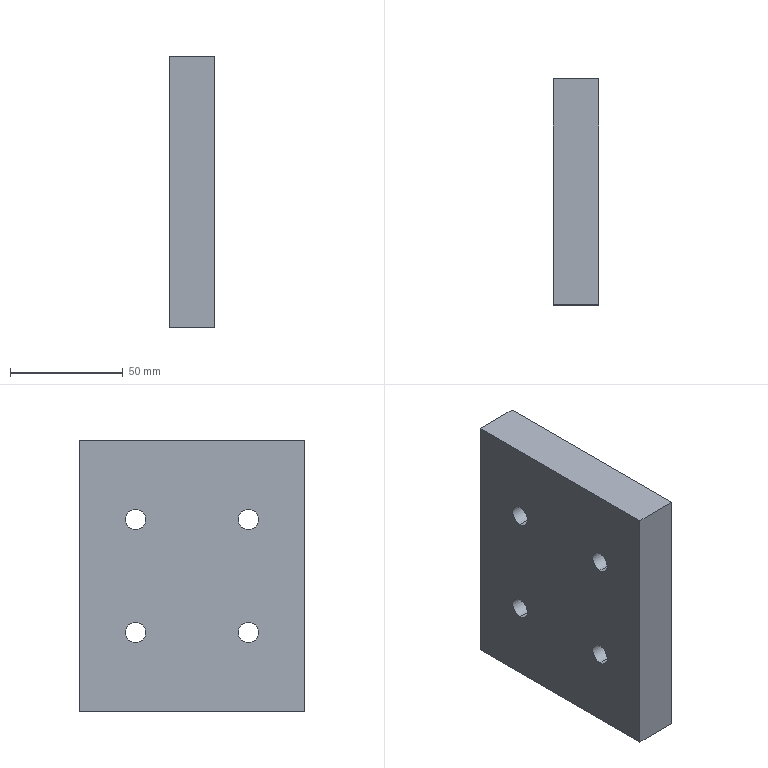Part | SolidWorks | features Extrusion 1, HoleWzd 1 | 1 solid | 14 faces | box 20 x 100 x 120 mm | volume 234911 mm3 | cylinder 8 | plane 6 | commonest cylinder face diameters 9 x8
STEP:
#1=CARTESIAN_POINT('',(0.,25.,29.5));
#2=VERTEX_POINT('',#1);
#3=CARTESIAN_POINT('',(0.,25.,20.5));
#4=VERTEX_POINT('',#3);
#5=CARTESIAN_POINT('',(0.,25.,25.));
#6=DIRECTION('',(1.,0.,0.));
#7=DIRECTION('',(0.,0.,-1.));
#8=AXIS2_PLACEMENT_3D('',#5,#6,#7);
#9=CIRCLE('',#8,4.5);
#10=EDGE_CURVE('',#2,#4,#9,.T.);
#11=ORIENTED_EDGE('',*,*,#10,.F.);
#12=CARTESIAN_POINT('',(20.,25.,29.5));
#13=VERTEX_POINT('',#12);
#14=CARTESIAN_POINT('',(20.,25.,29.5));
#15=DIRECTION('',(1.,0.,0.));
#16=VECTOR('',#15,1000.);
#17=LINE('',#14,#16);
#18=EDGE_CURVE('',#2,#13,#17,.T.);
#19=ORIENTED_EDGE('',*,*,#18,.T.);
#20=CARTESIAN_POINT('',(20.,25.,20.5));
#21=VERTEX_POINT('',#20);
#22=CARTESIAN_POINT('',(20.,25.,25.));
#23=DIRECTION('',(1.,0.,0.));
#24=DIRECTION('',(0.,0.,-1.));
#25=AXIS2_PLACEMENT_3D('',#22,#23,#24);
#26=CIRCLE('',#25,4.5);
#27=EDGE_CURVE('',#13,#21,#26,.T.);
#28=ORIENTED_EDGE('',*,*,#27,.T.);
#29=CARTESIAN_POINT('',(20.,25.,20.5));
#30=DIRECTION('',(1.,0.,0.));
#31=VECTOR('',#30,1000.);
#32=LINE('',#29,#31);
#33=EDGE_CURVE('',#4,#21,#32,.T.);
#34=ORIENTED_EDGE('',*,*,#33,.F.);
#35=EDGE_LOOP('',(#11,#19,#28,#34));
#36=FACE_OUTER_BOUND('',#35,.T.);
#37=CARTESIAN_POINT('',(20.,25.,25.));
#38=DIRECTION('',(1.,0.,0.));
#39=DIRECTION('',(0.,0.,-1.));
#40=AXIS2_PLACEMENT_3D('',#37,#38,#39);
#41=CYLINDRICAL_SURFACE('',#40,4.5);
#42=ADVANCED_FACE('',(#36),#41,.F.);
#43=CARTESIAN_POINT('',(0.,25.,-20.5));
#44=VERTEX_POINT('',#43);
#45=CARTESIAN_POINT('',(0.,25.,-29.5));
#46=VERTEX_POINT('',#45);
#47=CARTESIAN_POINT('',(0.,25.,-25.));
#48=DIRECTION('',(1.,0.,0.));
#49=DIRECTION('',(0.,0.,-1.));
#50=AXIS2_PLACEMENT_3D('',#47,#48,#49);
#51=CIRCLE('',#50,4.5);
#52=EDGE_CURVE('',#44,#46,#51,.T.);
#53=ORIENTED_EDGE('',*,*,#52,.F.);
#54=CARTESIAN_POINT('',(20.,25.,-20.5));
#55=VERTEX_POINT('',#54);
#56=CARTESIAN_POINT('',(20.,25.,-20.5));
#57=DIRECTION('',(1.,0.,0.));
#58=VECTOR('',#57,1000.);
#59=LINE('',#56,#58);
#60=EDGE_CURVE('',#44,#55,#59,.T.);
#61=ORIENTED_EDGE('',*,*,#60,.T.);
#62=CARTESIAN_POINT('',(20.,25.,-29.5));
#63=VERTEX_POINT('',#62);
#64=CARTESIAN_POINT('',(20.,25.,-25.));
#65=DIRECTION('',(1.,0.,0.));
#66=DIRECTION('',(0.,0.,-1.));
#67=AXIS2_PLACEMENT_3D('',#64,#65,#66);
#68=CIRCLE('',#67,4.5);
#69=EDGE_CURVE('',#55,#63,#68,.T.);
#70=ORIENTED_EDGE('',*,*,#69,.T.);
#71=CARTESIAN_POINT('',(20.,25.,-29.5));
#72=DIRECTION('',(1.,0.,0.));
#73=VECTOR('',#72,1000.);
#74=LINE('',#71,#73);
#75=EDGE_CURVE('',#46,#63,#74,.T.);
#76=ORIENTED_EDGE('',*,*,#75,.F.);
#77=EDGE_LOOP('',(#53,#61,#70,#76));
#78=FACE_OUTER_BOUND('',#77,.T.);
#79=CARTESIAN_POINT('',(20.,25.,-25.));
#80=DIRECTION('',(1.,0.,0.));
#81=DIRECTION('',(0.,0.,-1.));
#82=AXIS2_PLACEMENT_3D('',#79,#80,#81);
#83=CYLINDRICAL_SURFACE('',#82,4.5);
#84=ADVANCED_FACE('',(#78),#83,.F.);
#85=CARTESIAN_POINT('',(0.,-25.,29.5));
#86=VERTEX_POINT('',#85);
#87=CARTESIAN_POINT('',(0.,-25.,20.5));
#88=VERTEX_POINT('',#87);
#89=CARTESIAN_POINT('',(0.,-25.,25.));
#90=DIRECTION('',(1.,0.,0.));
#91=DIRECTION('',(0.,0.,-1.));
#92=AXIS2_PLACEMENT_3D('',#89,#90,#91);
#93=CIRCLE('',#92,4.5);
#94=EDGE_CURVE('',#86,#88,#93,.T.);
#95=ORIENTED_EDGE('',*,*,#94,.F.);
#96=CARTESIAN_POINT('',(20.,-25.,29.5));
#97=VERTEX_POINT('',#96);
#98=CARTESIAN_POINT('',(20.,-25.,29.5));
#99=DIRECTION('',(1.,0.,0.));
#100=VECTOR('',#99,1000.);
#101=LINE('',#98,#100);
#102=EDGE_CURVE('',#86,#97,#101,.T.);
#103=ORIENTED_EDGE('',*,*,#102,.T.);
#104=CARTESIAN_POINT('',(20.,-25.,20.5));
#105=VERTEX_POINT('',#104);
#106=CARTESIAN_POINT('',(20.,-25.,25.));
#107=DIRECTION('',(1.,0.,0.));
#108=DIRECTION('',(0.,0.,-1.));
#109=AXIS2_PLACEMENT_3D('',#106,#107,#108);
#110=CIRCLE('',#109,4.5);
#111=EDGE_CURVE('',#97,#105,#110,.T.);
#112=ORIENTED_EDGE('',*,*,#111,.T.);
#113=CARTESIAN_POINT('',(20.,-25.,20.5));
#114=DIRECTION('',(1.,0.,0.));
#115=VECTOR('',#114,1000.);
#116=LINE('',#113,#115);
#117=EDGE_CURVE('',#88,#105,#116,.T.);
#118=ORIENTED_EDGE('',*,*,#117,.F.);
#119=EDGE_LOOP('',(#95,#103,#112,#118));
#120=FACE_OUTER_BOUND('',#119,.T.);
#121=CARTESIAN_POINT('',(20.,-25.,25.));
#122=DIRECTION('',(1.,0.,0.));
#123=DIRECTION('',(0.,0.,-1.));
#124=AXIS2_PLACEMENT_3D('',#121,#122,#123);
#125=CYLINDRICAL_SURFACE('',#124,4.5);
#126=ADVANCED_FACE('',(#120),#125,.F.);
#127=CARTESIAN_POINT('',(0.,-25.,-20.5));
#128=VERTEX_POINT('',#127);
#129=CARTESIAN_POINT('',(0.,-25.,-29.5));
#130=VERTEX_POINT('',#129);
#131=CARTESIAN_POINT('',(0.,-25.,-25.));
#132=DIRECTION('',(1.,0.,0.));
#133=DIRECTION('',(0.,0.,-1.));
#134=AXIS2_PLACEMENT_3D('',#131,#132,#133);
#135=CIRCLE('',#134,4.5);
#136=EDGE_CURVE('',#128,#130,#135,.T.);
#137=ORIENTED_EDGE('',*,*,#136,.F.);
#138=CARTESIAN_POINT('',(20.,-25.,-20.5));
#139=VERTEX_POINT('',#138);
#140=CARTESIAN_POINT('',(20.,-25.,-20.5));
#141=DIRECTION('',(1.,0.,0.));
#142=VECTOR('',#141,1000.);
#143=LINE('',#140,#142);
#144=EDGE_CURVE('',#128,#139,#143,.T.);
#145=ORIENTED_EDGE('',*,*,#144,.T.);
#146=CARTESIAN_POINT('',(20.,-25.,-29.5));
#147=VERTEX_POINT('',#146);
#148=CARTESIAN_POINT('',(20.,-25.,-25.));
#149=DIRECTION('',(1.,0.,0.));
#150=DIRECTION('',(0.,0.,-1.));
#151=AXIS2_PLACEMENT_3D('',#148,#149,#150);
#152=CIRCLE('',#151,4.5);
#153=EDGE_CURVE('',#139,#147,#152,.T.);
#154=ORIENTED_EDGE('',*,*,#153,.T.);
#155=CARTESIAN_POINT('',(20.,-25.,-29.5));
#156=DIRECTION('',(1.,0.,0.));
#157=VECTOR('',#156,1000.);
#158=LINE('',#155,#157);
#159=EDGE_CURVE('',#130,#147,#158,.T.);
#160=ORIENTED_EDGE('',*,*,#159,.F.);
#161=EDGE_LOOP('',(#137,#145,#154,#160));
#162=FACE_OUTER_BOUND('',#161,.T.);
#163=CARTESIAN_POINT('',(20.,-25.,-25.));
#164=DIRECTION('',(1.,0.,0.));
#165=DIRECTION('',(0.,0.,-1.));
#166=AXIS2_PLACEMENT_3D('',#163,#164,#165);
#167=CYLINDRICAL_SURFACE('',#166,4.5);
#168=ADVANCED_FACE('',(#162),#167,.F.);
#169=CARTESIAN_POINT('',(0.,-50.,-60.));
#170=VERTEX_POINT('',#169);
#171=CARTESIAN_POINT('',(0.,50.,-60.));
#172=VERTEX_POINT('',#171);
#173=CARTESIAN_POINT('',(0.,50.,-60.));
#174=DIRECTION('',(0.,1.,0.));
#175=VECTOR('',#174,1000.);
#176=LINE('',#173,#175);
#177=EDGE_CURVE('',#170,#172,#176,.T.);
#178=ORIENTED_EDGE('',*,*,#177,.T.);
#179=CARTESIAN_POINT('',(20.,50.,-60.));
#180=VERTEX_POINT('',#179);
#181=CARTESIAN_POINT('',(20.,50.,-60.));
#182=DIRECTION('',(-1.,0.,0.));
#183=VECTOR('',#182,1000.);
#184=LINE('',#181,#183);
#185=EDGE_CURVE('',#180,#172,#184,.T.);
#186=ORIENTED_EDGE('',*,*,#185,.F.);
#187=CARTESIAN_POINT('',(20.,-50.,-60.));
#188=VERTEX_POINT('',#187);
#189=CARTESIAN_POINT('',(20.,50.,-60.));
#190=DIRECTION('',(0.,1.,0.));
#191=VECTOR('',#190,1000.);
#192=LINE('',#189,#191);
#193=EDGE_CURVE('',#188,#180,#192,.T.);
#194=ORIENTED_EDGE('',*,*,#193,.F.);
#195=CARTESIAN_POINT('',(20.,-50.,-60.));
#196=DIRECTION('',(-1.,0.,0.));
#197=VECTOR('',#196,1000.);
#198=LINE('',#195,#197);
#199=EDGE_CURVE('',#188,#170,#198,.T.);
#200=ORIENTED_EDGE('',*,*,#199,.T.);
#201=EDGE_LOOP('',(#178,#186,#194,#200));
#202=FACE_OUTER_BOUND('',#201,.T.);
#203=CARTESIAN_POINT('',(20.,50.,-60.));
#204=DIRECTION('',(0.,0.,1.));
#205=DIRECTION('',(0.,-1.,0.));
#206=AXIS2_PLACEMENT_3D('',#203,#204,#205);
#207=PLANE('',#206);
#208=ADVANCED_FACE('',(#202),#207,.F.);
#209=CARTESIAN_POINT('',(0.,50.,60.));
#210=VERTEX_POINT('',#209);
#211=CARTESIAN_POINT('',(0.,50.,60.));
#212=DIRECTION('',(0.,0.,1.));
#213=VECTOR('',#212,1000.);
#214=LINE('',#211,#213);
#215=EDGE_CURVE('',#172,#210,#214,.T.);
#216=ORIENTED_EDGE('',*,*,#215,.T.);
#217=CARTESIAN_POINT('',(20.,50.,60.));
#218=VERTEX_POINT('',#217);
#219=CARTESIAN_POINT('',(20.,50.,60.));
#220=DIRECTION('',(-1.,0.,0.));
#221=VECTOR('',#220,1000.);
#222=LINE('',#219,#221);
#223=EDGE_CURVE('',#218,#210,#222,.T.);
#224=ORIENTED_EDGE('',*,*,#223,.F.);
#225=CARTESIAN_POINT('',(20.,50.,60.));
#226=DIRECTION('',(0.,0.,1.));
#227=VECTOR('',#226,1000.);
#228=LINE('',#225,#227);
#229=EDGE_CURVE('',#180,#218,#228,.T.);
#230=ORIENTED_EDGE('',*,*,#229,.F.);
#231=ORIENTED_EDGE('',*,*,#185,.T.);
#232=EDGE_LOOP('',(#216,#224,#230,#231));
#233=FACE_OUTER_BOUND('',#232,.T.);
#234=CARTESIAN_POINT('',(20.,50.,60.));
#235=DIRECTION('',(0.,-1.,0.));
#236=DIRECTION('',(0.,0.,-1.));
#237=AXIS2_PLACEMENT_3D('',#234,#235,#236);
#238=PLANE('',#237);
#239=ADVANCED_FACE('',(#233),#238,.F.);
#240=CARTESIAN_POINT('',(0.,-50.,60.));
#241=VERTEX_POINT('',#240);
#242=CARTESIAN_POINT('',(0.,50.,60.));
#243=DIRECTION('',(0.,-1.,0.));
#244=VECTOR('',#243,1000.);
#245=LINE('',#242,#244);
#246=EDGE_CURVE('',#210,#241,#245,.T.);
#247=ORIENTED_EDGE('',*,*,#246,.T.);
#248=CARTESIAN_POINT('',(20.,-50.,60.));
#249=VERTEX_POINT('',#248);
#250=CARTESIAN_POINT('',(20.,-50.,60.));
#251=DIRECTION('',(-1.,0.,0.));
#252=VECTOR('',#251,1000.);
#253=LINE('',#250,#252);
#254=EDGE_CURVE('',#249,#241,#253,.T.);
#255=ORIENTED_EDGE('',*,*,#254,.F.);
#256=CARTESIAN_POINT('',(20.,50.,60.));
#257=DIRECTION('',(0.,-1.,0.));
#258=VECTOR('',#257,1000.);
#259=LINE('',#256,#258);
#260=EDGE_CURVE('',#218,#249,#259,.T.);
#261=ORIENTED_EDGE('',*,*,#260,.F.);
#262=ORIENTED_EDGE('',*,*,#223,.T.);
#263=EDGE_LOOP('',(#247,#255,#261,#262));
#264=FACE_OUTER_BOUND('',#263,.T.);
#265=CARTESIAN_POINT('',(20.,50.,60.));
#266=DIRECTION('',(0.,0.,-1.));
#267=DIRECTION('',(0.,1.,0.));
#268=AXIS2_PLACEMENT_3D('',#265,#266,#267);
#269=PLANE('',#268);
#270=ADVANCED_FACE('',(#264),#269,.F.);
#271=CARTESIAN_POINT('',(0.,-50.,60.));
#272=DIRECTION('',(0.,0.,-1.));
#273=VECTOR('',#272,1000.);
#274=LINE('',#271,#273);
#275=EDGE_CURVE('',#241,#170,#274,.T.);
#276=ORIENTED_EDGE('',*,*,#275,.T.);
#277=ORIENTED_EDGE('',*,*,#199,.F.);
#278=CARTESIAN_POINT('',(20.,-50.,60.));
#279=DIRECTION('',(0.,0.,-1.));
#280=VECTOR('',#279,1000.);
#281=LINE('',#278,#280);
#282=EDGE_CURVE('',#249,#188,#281,.T.);
#283=ORIENTED_EDGE('',*,*,#282,.F.);
#284=ORIENTED_EDGE('',*,*,#254,.T.);
#285=EDGE_LOOP('',(#276,#277,#283,#284));
#286=FACE_OUTER_BOUND('',#285,.T.);
#287=CARTESIAN_POINT('',(20.,-50.,60.));
#288=DIRECTION('',(0.,1.,0.));
#289=DIRECTION('',(0.,0.,1.));
#290=AXIS2_PLACEMENT_3D('',#287,#288,#289);
#291=PLANE('',#290);
#292=ADVANCED_FACE('',(#286),#291,.F.);
#293=CARTESIAN_POINT('',(20.,25.,25.));
#294=DIRECTION('',(1.,0.,0.));
#295=DIRECTION('',(0.,0.,-1.));
#296=AXIS2_PLACEMENT_3D('',#293,#294,#295);
#297=CIRCLE('',#296,4.5);
#298=EDGE_CURVE('',#21,#13,#297,.T.);
#299=ORIENTED_EDGE('',*,*,#298,.F.);
#300=ORIENTED_EDGE('',*,*,#27,.F.);
#301=EDGE_LOOP('',(#299,#300));
#302=FACE_BOUND('',#301,.T.);
#303=CARTESIAN_POINT('',(20.,25.,-25.));
#304=DIRECTION('',(1.,0.,0.));
#305=DIRECTION('',(0.,0.,-1.));
#306=AXIS2_PLACEMENT_3D('',#303,#304,#305);
#307=CIRCLE('',#306,4.5);
#308=EDGE_CURVE('',#63,#55,#307,.T.);
#309=ORIENTED_EDGE('',*,*,#308,.F.);
#310=ORIENTED_EDGE('',*,*,#69,.F.);
#311=EDGE_LOOP('',(#309,#310));
#312=FACE_BOUND('',#311,.T.);
#313=CARTESIAN_POINT('',(20.,-25.,25.));
#314=DIRECTION('',(1.,0.,0.));
#315=DIRECTION('',(0.,0.,-1.));
#316=AXIS2_PLACEMENT_3D('',#313,#314,#315);
#317=CIRCLE('',#316,4.5);
#318=EDGE_CURVE('',#105,#97,#317,.T.);
#319=ORIENTED_EDGE('',*,*,#318,.F.);
#320=ORIENTED_EDGE('',*,*,#111,.F.);
#321=EDGE_LOOP('',(#319,#320));
#322=FACE_BOUND('',#321,.T.);
#323=CARTESIAN_POINT('',(20.,-25.,-25.));
#324=DIRECTION('',(1.,0.,0.));
#325=DIRECTION('',(0.,0.,-1.));
#326=AXIS2_PLACEMENT_3D('',#323,#324,#325);
#327=CIRCLE('',#326,4.5);
#328=EDGE_CURVE('',#147,#139,#327,.T.);
#329=ORIENTED_EDGE('',*,*,#328,.F.);
#330=ORIENTED_EDGE('',*,*,#153,.F.);
#331=EDGE_LOOP('',(#329,#330));
#332=FACE_BOUND('',#331,.T.);
#333=ORIENTED_EDGE('',*,*,#193,.T.);
#334=ORIENTED_EDGE('',*,*,#229,.T.);
#335=ORIENTED_EDGE('',*,*,#260,.T.);
#336=ORIENTED_EDGE('',*,*,#282,.T.);
#337=EDGE_LOOP('',(#333,#334,#335,#336));
#338=FACE_OUTER_BOUND('',#337,.T.);
#339=CARTESIAN_POINT('',(20.,0.,0.));
#340=DIRECTION('',(1.,0.,0.));
#341=DIRECTION('',(0.,0.,-1.));
#342=AXIS2_PLACEMENT_3D('',#339,#340,#341);
#343=PLANE('',#342);
#344=ADVANCED_FACE('',(#302,#312,#322,#332,#338),#343,.T.);
#345=CARTESIAN_POINT('',(0.,25.,25.));
#346=DIRECTION('',(1.,0.,0.));
#347=DIRECTION('',(0.,0.,-1.));
#348=AXIS2_PLACEMENT_3D('',#345,#346,#347);
#349=CIRCLE('',#348,4.5);
#350=EDGE_CURVE('',#4,#2,#349,.T.);
#351=ORIENTED_EDGE('',*,*,#350,.T.);
#352=ORIENTED_EDGE('',*,*,#10,.T.);
#353=EDGE_LOOP('',(#351,#352));
#354=FACE_BOUND('',#353,.T.);
#355=CARTESIAN_POINT('',(0.,25.,-25.));
#356=DIRECTION('',(1.,0.,0.));
#357=DIRECTION('',(0.,0.,-1.));
#358=AXIS2_PLACEMENT_3D('',#355,#356,#357);
#359=CIRCLE('',#358,4.5);
#360=EDGE_CURVE('',#46,#44,#359,.T.);
#361=ORIENTED_EDGE('',*,*,#360,.T.);
#362=ORIENTED_EDGE('',*,*,#52,.T.);
#363=EDGE_LOOP('',(#361,#362));
#364=FACE_BOUND('',#363,.T.);
#365=CARTESIAN_POINT('',(0.,-25.,25.));
#366=DIRECTION('',(1.,0.,0.));
#367=DIRECTION('',(0.,0.,-1.));
#368=AXIS2_PLACEMENT_3D('',#365,#366,#367);
#369=CIRCLE('',#368,4.5);
#370=EDGE_CURVE('',#88,#86,#369,.T.);
#371=ORIENTED_EDGE('',*,*,#370,.T.);
#372=ORIENTED_EDGE('',*,*,#94,.T.);
#373=EDGE_LOOP('',(#371,#372));
#374=FACE_BOUND('',#373,.T.);
#375=CARTESIAN_POINT('',(0.,-25.,-25.));
#376=DIRECTION('',(1.,0.,0.));
#377=DIRECTION('',(0.,0.,-1.));
#378=AXIS2_PLACEMENT_3D('',#375,#376,#377);
#379=CIRCLE('',#378,4.5);
#380=EDGE_CURVE('',#130,#128,#379,.T.);
#381=ORIENTED_EDGE('',*,*,#380,.T.);
#382=ORIENTED_EDGE('',*,*,#136,.T.);
#383=EDGE_LOOP('',(#381,#382));
#384=FACE_BOUND('',#383,.T.);
#385=ORIENTED_EDGE('',*,*,#177,.F.);
#386=ORIENTED_EDGE('',*,*,#275,.F.);
#387=ORIENTED_EDGE('',*,*,#246,.F.);
#388=ORIENTED_EDGE('',*,*,#215,.F.);
#389=EDGE_LOOP('',(#385,#386,#387,#388));
#390=FACE_OUTER_BOUND('',#389,.T.);
#391=CARTESIAN_POINT('',(0.,0.,0.));
#392=DIRECTION('',(1.,0.,0.));
#393=DIRECTION('',(0.,0.,-1.));
#394=AXIS2_PLACEMENT_3D('',#391,#392,#393);
#395=PLANE('',#394);
#396=ADVANCED_FACE('',(#354,#364,#374,#384,#390),#395,.F.);
#397=ORIENTED_EDGE('',*,*,#144,.F.);
#398=ORIENTED_EDGE('',*,*,#380,.F.);
#399=ORIENTED_EDGE('',*,*,#159,.T.);
#400=ORIENTED_EDGE('',*,*,#328,.T.);
#401=EDGE_LOOP('',(#397,#398,#399,#400));
#402=FACE_OUTER_BOUND('',#401,.T.);
#403=CARTESIAN_POINT('',(20.,-25.,-25.));
#404=DIRECTION('',(1.,0.,0.));
#405=DIRECTION('',(0.,0.,-1.));
#406=AXIS2_PLACEMENT_3D('',#403,#404,#405);
#407=CYLINDRICAL_SURFACE('',#406,4.5);
#408=ADVANCED_FACE('',(#402),#407,.F.);
#409=ORIENTED_EDGE('',*,*,#102,.F.);
#410=ORIENTED_EDGE('',*,*,#370,.F.);
#411=ORIENTED_EDGE('',*,*,#117,.T.);
#412=ORIENTED_EDGE('',*,*,#318,.T.);
#413=EDGE_LOOP('',(#409,#410,#411,#412));
#414=FACE_OUTER_BOUND('',#413,.T.);
#415=CARTESIAN_POINT('',(20.,-25.,25.));
#416=DIRECTION('',(1.,0.,0.));
#417=DIRECTION('',(0.,0.,-1.));
#418=AXIS2_PLACEMENT_3D('',#415,#416,#417);
#419=CYLINDRICAL_SURFACE('',#418,4.5);
#420=ADVANCED_FACE('',(#414),#419,.F.);
#421=ORIENTED_EDGE('',*,*,#60,.F.);
#422=ORIENTED_EDGE('',*,*,#360,.F.);
#423=ORIENTED_EDGE('',*,*,#75,.T.);
#424=ORIENTED_EDGE('',*,*,#308,.T.);
#425=EDGE_LOOP('',(#421,#422,#423,#424));
#426=FACE_OUTER_BOUND('',#425,.T.);
#427=CARTESIAN_POINT('',(20.,25.,-25.));
#428=DIRECTION('',(1.,0.,0.));
#429=DIRECTION('',(0.,0.,-1.));
#430=AXIS2_PLACEMENT_3D('',#427,#428,#429);
#431=CYLINDRICAL_SURFACE('',#430,4.5);
#432=ADVANCED_FACE('',(#426),#431,.F.);
#433=ORIENTED_EDGE('',*,*,#18,.F.);
#434=ORIENTED_EDGE('',*,*,#350,.F.);
#435=ORIENTED_EDGE('',*,*,#33,.T.);
#436=ORIENTED_EDGE('',*,*,#298,.T.);
#437=EDGE_LOOP('',(#433,#434,#435,#436));
#438=FACE_OUTER_BOUND('',#437,.T.);
#439=CARTESIAN_POINT('',(20.,25.,25.));
#440=DIRECTION('',(1.,0.,0.));
#441=DIRECTION('',(0.,0.,-1.));
#442=AXIS2_PLACEMENT_3D('',#439,#440,#441);
#443=CYLINDRICAL_SURFACE('',#442,4.5);
#444=ADVANCED_FACE('',(#438),#443,.F.);
#445=CLOSED_SHELL('',(#42,#84,#126,#168,#208,#239,#270,#292,#344,#396,#408,#420,#432,#444));
#446=MANIFOLD_SOLID_BREP('',#445);
#447=CARTESIAN_POINT('',(0.,0.,0.));
#448=DIRECTION('',(0.,0.,1.));
#449=DIRECTION('',(1.,0.,0.));
#450=AXIS2_PLACEMENT_3D('',#447,#448,#449);
#451=(LENGTH_UNIT()NAMED_UNIT(*)SI_UNIT(.MILLI.,.METRE.));
#452=UNCERTAINTY_MEASURE_WITH_UNIT(LENGTH_MEASURE(0.00001),#451,'','');
#453=(NAMED_UNIT(*)PLANE_ANGLE_UNIT()SI_UNIT($,.RADIAN.));
#454=(NAMED_UNIT(*)SI_UNIT($,.STERADIAN.)SOLID_ANGLE_UNIT());
#455=(GEOMETRIC_REPRESENTATION_CONTEXT(3)GLOBAL_UNCERTAINTY_ASSIGNED_CONTEXT((#452))GLOBAL_UNIT_ASSIGNED_CONTEXT((#451,#453,#454))REPRESENTATION_CONTEXT('',''));
#456=ADVANCED_BREP_SHAPE_REPRESENTATION('',(#446,#450),#455);